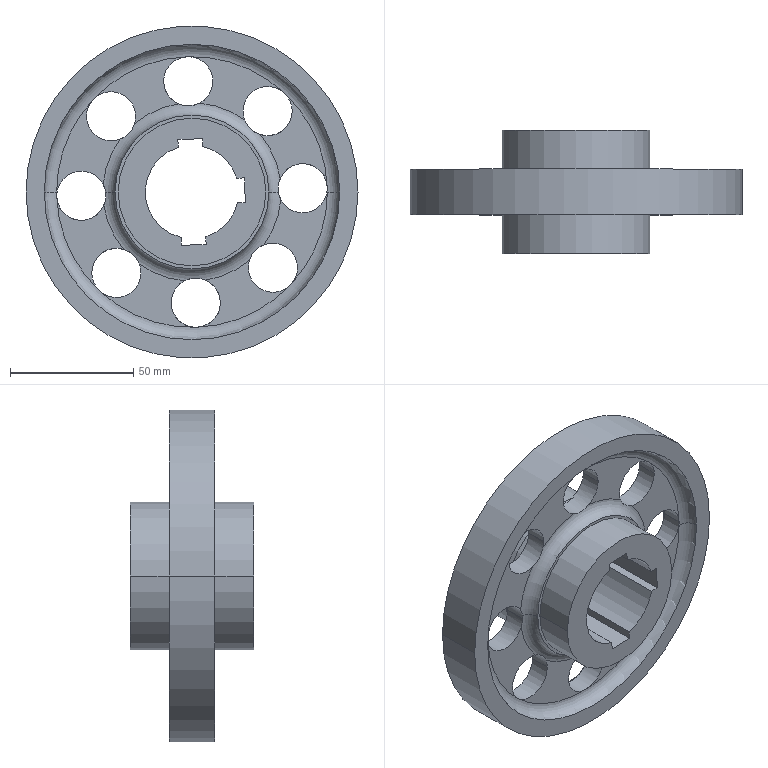Part | STEP file | 2026.6.15-Main Assembly图.sldasm-Part-119 | 1 solid | 59 faces | box 134.9 x 50 x 134.9 mm | volume 194237 mm3 | cylinder 27 | plane 24 | torus 8 | commonest cylinder face diameters 20 x16 60 x4 38 x3 62.5 x2 134.9 x2